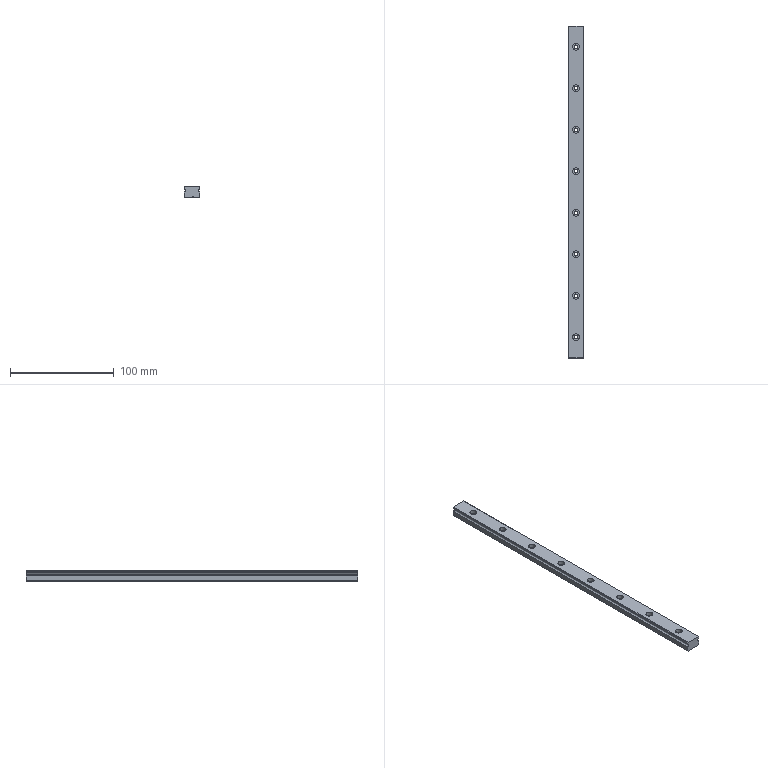Part | SolidWorks | features BaseBody 1 | 1 solid | 65 faces | box 15 x 320 x 10 mm | volume 44223 mm3 | cylinder 44 | plane 21 | commonest cylinder face diameters 3.4 x17 6.5 x17 0.6 x7 3 x3